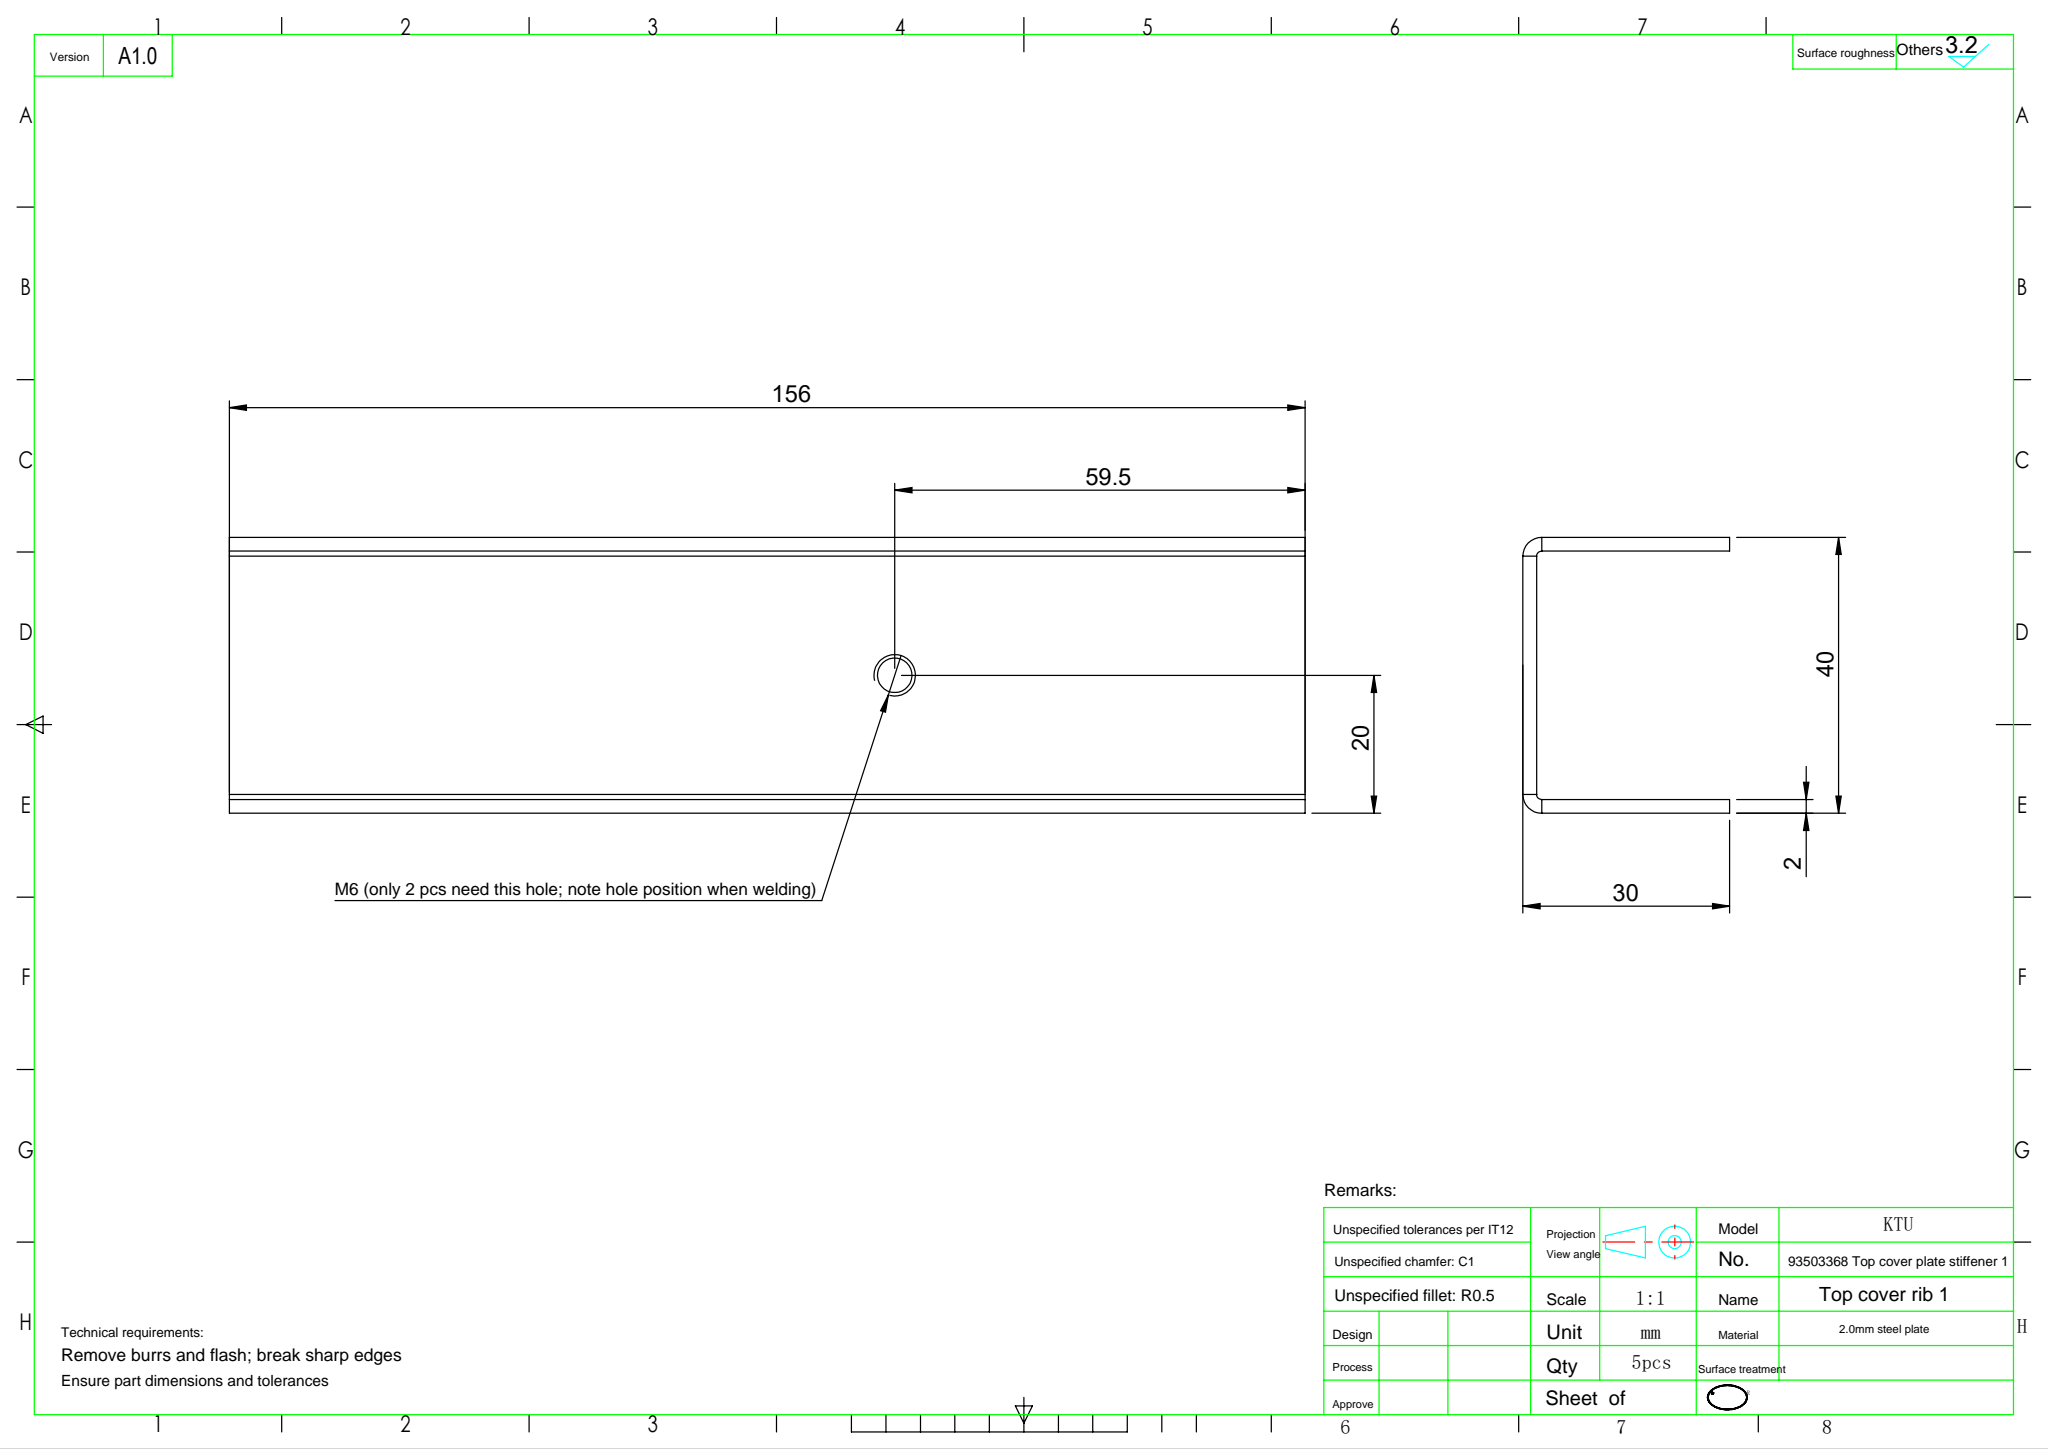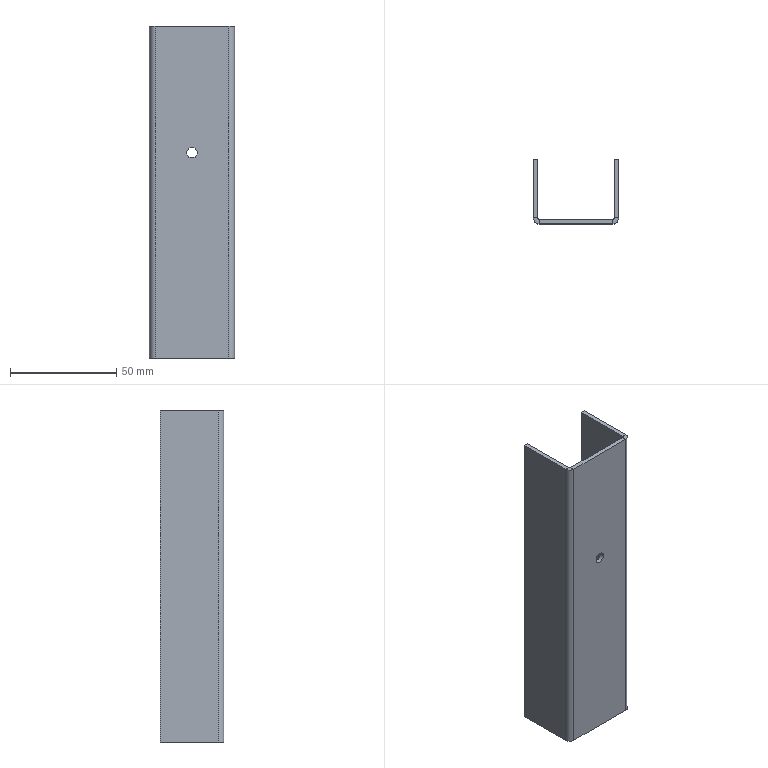Part | SolidWorks | features Cut 1, FlatPattern 1, SMBaseFlange 1, SheetMetal 1 | 1 solid | 24 faces | box 40 x 30 x 156 mm | volume 29448 mm3 | plane 18 | cylinder 6 | commonest cylinder face diameters 1.473 x2 5 x2 5.473 x2
STEP:
#1=CARTESIAN_POINT('',(2.5,-15.,18.5));
#2=VERTEX_POINT('',#1);
#3=CARTESIAN_POINT('',(-2.5,-15.,18.5));
#4=VERTEX_POINT('',#3);
#5=CARTESIAN_POINT('',(0.,-15.,18.5));
#6=DIRECTION('',(0.,1.,0.));
#7=DIRECTION('',(-1.,0.,0.));
#8=AXIS2_PLACEMENT_3D('',#5,#6,#7);
#9=CIRCLE('',#8,2.5);
#10=EDGE_CURVE('',#2,#4,#9,.T.);
#11=ORIENTED_EDGE('',*,*,#10,.F.);
#12=CARTESIAN_POINT('',(2.5,-13.,18.5));
#13=VERTEX_POINT('',#12);
#14=CARTESIAN_POINT('',(2.5,-23.,18.5));
#15=DIRECTION('',(0.,1.,0.));
#16=VECTOR('',#15,1000.);
#17=LINE('',#14,#16);
#18=EDGE_CURVE('',#2,#13,#17,.T.);
#19=ORIENTED_EDGE('',*,*,#18,.T.);
#20=CARTESIAN_POINT('',(-2.5,-13.,18.5));
#21=VERTEX_POINT('',#20);
#22=CARTESIAN_POINT('',(0.,-13.,18.5));
#23=DIRECTION('',(0.,1.,0.));
#24=DIRECTION('',(-1.,0.,0.));
#25=AXIS2_PLACEMENT_3D('',#22,#23,#24);
#26=CIRCLE('',#25,2.5);
#27=EDGE_CURVE('',#13,#21,#26,.T.);
#28=ORIENTED_EDGE('',*,*,#27,.T.);
#29=CARTESIAN_POINT('',(-2.5,-23.,18.5));
#30=DIRECTION('',(0.,1.,0.));
#31=VECTOR('',#30,1000.);
#32=LINE('',#29,#31);
#33=EDGE_CURVE('',#4,#21,#32,.T.);
#34=ORIENTED_EDGE('',*,*,#33,.F.);
#35=EDGE_LOOP('',(#11,#19,#28,#34));
#36=FACE_OUTER_BOUND('',#35,.T.);
#37=CARTESIAN_POINT('',(0.,-23.,18.5));
#38=DIRECTION('',(0.,1.,0.));
#39=DIRECTION('',(-1.,0.,0.));
#40=AXIS2_PLACEMENT_3D('',#37,#38,#39);
#41=CYLINDRICAL_SURFACE('',#40,2.5);
#42=ADVANCED_FACE('',(#36),#41,.F.);
#43=CARTESIAN_POINT('',(-20.,-12.263,78.));
#44=VERTEX_POINT('',#43);
#45=CARTESIAN_POINT('',(-18.,-12.263,78.));
#46=VERTEX_POINT('',#45);
#47=CARTESIAN_POINT('',(-20.,-12.263,78.));
#48=DIRECTION('',(1.,0.,0.));
#49=VECTOR('',#48,1000.);
#50=LINE('',#47,#49);
#51=EDGE_CURVE('',#44,#46,#50,.T.);
#52=ORIENTED_EDGE('',*,*,#51,.F.);
#53=CARTESIAN_POINT('',(-17.263,-15.,78.));
#54=VERTEX_POINT('',#53);
#55=CARTESIAN_POINT('',(-17.263,-12.263,78.));
#56=DIRECTION('',(0.,0.,1.));
#57=DIRECTION('',(-1.,0.,0.));
#58=AXIS2_PLACEMENT_3D('',#55,#56,#57);
#59=CIRCLE('',#58,2.737);
#60=EDGE_CURVE('',#44,#54,#59,.T.);
#61=ORIENTED_EDGE('',*,*,#60,.T.);
#62=CARTESIAN_POINT('',(-17.263,-13.,78.));
#63=VERTEX_POINT('',#62);
#64=CARTESIAN_POINT('',(-17.263,-13.,78.));
#65=DIRECTION('',(0.,-1.,0.));
#66=VECTOR('',#65,1000.);
#67=LINE('',#64,#66);
#68=EDGE_CURVE('',#63,#54,#67,.T.);
#69=ORIENTED_EDGE('',*,*,#68,.F.);
#70=CARTESIAN_POINT('',(-17.263,-12.263,78.));
#71=DIRECTION('',(0.,0.,1.));
#72=DIRECTION('',(1.,0.,0.));
#73=AXIS2_PLACEMENT_3D('',#70,#71,#72);
#74=CIRCLE('',#73,0.7366);
#75=EDGE_CURVE('',#46,#63,#74,.T.);
#76=ORIENTED_EDGE('',*,*,#75,.F.);
#77=EDGE_LOOP('',(#52,#61,#69,#76));
#78=FACE_OUTER_BOUND('',#77,.T.);
#79=CARTESIAN_POINT('',(-20.,-12.263,78.));
#80=DIRECTION('',(0.,0.,1.));
#81=DIRECTION('',(1.,0.,0.));
#82=AXIS2_PLACEMENT_3D('',#79,#80,#81);
#83=PLANE('',#82);
#84=ADVANCED_FACE('',(#78),#83,.T.);
#85=CARTESIAN_POINT('',(-20.,15.,78.));
#86=VERTEX_POINT('',#85);
#87=CARTESIAN_POINT('',(-20.,-15.,78.));
#88=DIRECTION('',(0.,-1.,0.));
#89=VECTOR('',#88,1000.);
#90=LINE('',#87,#89);
#91=EDGE_CURVE('',#86,#44,#90,.T.);
#92=ORIENTED_EDGE('',*,*,#91,.T.);
#93=ORIENTED_EDGE('',*,*,#51,.T.);
#94=CARTESIAN_POINT('',(-18.,15.,78.));
#95=VERTEX_POINT('',#94);
#96=CARTESIAN_POINT('',(-18.,-15.,78.));
#97=DIRECTION('',(0.,-1.,0.));
#98=VECTOR('',#97,1000.);
#99=LINE('',#96,#98);
#100=EDGE_CURVE('',#95,#46,#99,.T.);
#101=ORIENTED_EDGE('',*,*,#100,.F.);
#102=CARTESIAN_POINT('',(-20.,15.,78.));
#103=DIRECTION('',(1.,0.,0.));
#104=VECTOR('',#103,1000.);
#105=LINE('',#102,#104);
#106=EDGE_CURVE('',#86,#95,#105,.T.);
#107=ORIENTED_EDGE('',*,*,#106,.F.);
#108=EDGE_LOOP('',(#92,#93,#101,#107));
#109=FACE_OUTER_BOUND('',#108,.T.);
#110=CARTESIAN_POINT('',(-17.263,-13.,78.));
#111=DIRECTION('',(0.,0.,1.));
#112=DIRECTION('',(1.,0.,0.));
#113=AXIS2_PLACEMENT_3D('',#110,#111,#112);
#114=PLANE('',#113);
#115=ADVANCED_FACE('',(#109),#114,.T.);
#116=CARTESIAN_POINT('',(-17.263,-15.,-78.));
#117=VERTEX_POINT('',#116);
#118=CARTESIAN_POINT('',(-17.263,-13.,-78.));
#119=VERTEX_POINT('',#118);
#120=CARTESIAN_POINT('',(-17.263,-15.,-78.));
#121=DIRECTION('',(0.,1.,0.));
#122=VECTOR('',#121,1000.);
#123=LINE('',#120,#122);
#124=EDGE_CURVE('',#117,#119,#123,.T.);
#125=ORIENTED_EDGE('',*,*,#124,.F.);
#126=CARTESIAN_POINT('',(-20.,-12.263,-78.));
#127=VERTEX_POINT('',#126);
#128=CARTESIAN_POINT('',(-17.263,-12.263,-78.));
#129=DIRECTION('',(0.,0.,1.));
#130=DIRECTION('',(-1.,0.,0.));
#131=AXIS2_PLACEMENT_3D('',#128,#129,#130);
#132=CIRCLE('',#131,2.737);
#133=EDGE_CURVE('',#127,#117,#132,.T.);
#134=ORIENTED_EDGE('',*,*,#133,.F.);
#135=CARTESIAN_POINT('',(-18.,-12.263,-78.));
#136=VERTEX_POINT('',#135);
#137=CARTESIAN_POINT('',(-18.,-12.263,-78.));
#138=DIRECTION('',(-1.,0.,0.));
#139=VECTOR('',#138,1000.);
#140=LINE('',#137,#139);
#141=EDGE_CURVE('',#136,#127,#140,.T.);
#142=ORIENTED_EDGE('',*,*,#141,.F.);
#143=CARTESIAN_POINT('',(-17.263,-12.263,-78.));
#144=DIRECTION('',(0.,0.,1.));
#145=DIRECTION('',(1.,0.,0.));
#146=AXIS2_PLACEMENT_3D('',#143,#144,#145);
#147=CIRCLE('',#146,0.7366);
#148=EDGE_CURVE('',#136,#119,#147,.T.);
#149=ORIENTED_EDGE('',*,*,#148,.T.);
#150=EDGE_LOOP('',(#125,#134,#142,#149));
#151=FACE_OUTER_BOUND('',#150,.T.);
#152=CARTESIAN_POINT('',(-17.263,-15.,-78.));
#153=DIRECTION('',(0.,0.,-1.));
#154=DIRECTION('',(-1.,0.,0.));
#155=AXIS2_PLACEMENT_3D('',#152,#153,#154);
#156=PLANE('',#155);
#157=ADVANCED_FACE('',(#151),#156,.T.);
#158=CARTESIAN_POINT('',(17.263,-15.,-78.));
#159=VERTEX_POINT('',#158);
#160=CARTESIAN_POINT('',(20.,-15.,-78.));
#161=DIRECTION('',(1.,0.,0.));
#162=VECTOR('',#161,1000.);
#163=LINE('',#160,#162);
#164=EDGE_CURVE('',#117,#159,#163,.T.);
#165=ORIENTED_EDGE('',*,*,#164,.F.);
#166=ORIENTED_EDGE('',*,*,#124,.T.);
#167=CARTESIAN_POINT('',(17.263,-13.,-78.));
#168=VERTEX_POINT('',#167);
#169=CARTESIAN_POINT('',(20.,-13.,-78.));
#170=DIRECTION('',(1.,0.,0.));
#171=VECTOR('',#170,1000.);
#172=LINE('',#169,#171);
#173=EDGE_CURVE('',#119,#168,#172,.T.);
#174=ORIENTED_EDGE('',*,*,#173,.T.);
#175=CARTESIAN_POINT('',(17.263,-13.,-78.));
#176=DIRECTION('',(0.,-1.,0.));
#177=VECTOR('',#176,1000.);
#178=LINE('',#175,#177);
#179=EDGE_CURVE('',#168,#159,#178,.T.);
#180=ORIENTED_EDGE('',*,*,#179,.T.);
#181=EDGE_LOOP('',(#165,#166,#174,#180));
#182=FACE_OUTER_BOUND('',#181,.T.);
#183=CARTESIAN_POINT('',(-18.,-12.263,-78.));
#184=DIRECTION('',(0.,0.,-1.));
#185=DIRECTION('',(-1.,0.,0.));
#186=AXIS2_PLACEMENT_3D('',#183,#184,#185);
#187=PLANE('',#186);
#188=ADVANCED_FACE('',(#182),#187,.T.);
#189=CARTESIAN_POINT('',(17.263,-15.,78.));
#190=VERTEX_POINT('',#189);
#191=CARTESIAN_POINT('',(17.263,-13.,78.));
#192=VERTEX_POINT('',#191);
#193=CARTESIAN_POINT('',(17.263,-15.,78.));
#194=DIRECTION('',(0.,1.,0.));
#195=VECTOR('',#194,1000.);
#196=LINE('',#193,#195);
#197=EDGE_CURVE('',#190,#192,#196,.T.);
#198=ORIENTED_EDGE('',*,*,#197,.F.);
#199=CARTESIAN_POINT('',(20.,-12.263,78.));
#200=VERTEX_POINT('',#199);
#201=CARTESIAN_POINT('',(17.263,-12.263,78.));
#202=DIRECTION('',(0.,0.,1.));
#203=DIRECTION('',(-1.,0.,0.));
#204=AXIS2_PLACEMENT_3D('',#201,#202,#203);
#205=CIRCLE('',#204,2.737);
#206=EDGE_CURVE('',#190,#200,#205,.T.);
#207=ORIENTED_EDGE('',*,*,#206,.T.);
#208=CARTESIAN_POINT('',(18.,-12.263,78.));
#209=VERTEX_POINT('',#208);
#210=CARTESIAN_POINT('',(18.,-12.263,78.));
#211=DIRECTION('',(1.,0.,0.));
#212=VECTOR('',#211,1000.);
#213=LINE('',#210,#212);
#214=EDGE_CURVE('',#209,#200,#213,.T.);
#215=ORIENTED_EDGE('',*,*,#214,.F.);
#216=CARTESIAN_POINT('',(17.263,-12.263,78.));
#217=DIRECTION('',(0.,0.,1.));
#218=DIRECTION('',(1.,0.,0.));
#219=AXIS2_PLACEMENT_3D('',#216,#217,#218);
#220=CIRCLE('',#219,0.7366);
#221=EDGE_CURVE('',#192,#209,#220,.T.);
#222=ORIENTED_EDGE('',*,*,#221,.F.);
#223=EDGE_LOOP('',(#198,#207,#215,#222));
#224=FACE_OUTER_BOUND('',#223,.T.);
#225=CARTESIAN_POINT('',(17.263,-15.,78.));
#226=DIRECTION('',(0.,0.,1.));
#227=DIRECTION('',(1.,0.,0.));
#228=AXIS2_PLACEMENT_3D('',#225,#226,#227);
#229=PLANE('',#228);
#230=ADVANCED_FACE('',(#224),#229,.T.);
#231=CARTESIAN_POINT('',(20.,-15.,78.));
#232=DIRECTION('',(1.,0.,0.));
#233=VECTOR('',#232,1000.);
#234=LINE('',#231,#233);
#235=EDGE_CURVE('',#54,#190,#234,.T.);
#236=ORIENTED_EDGE('',*,*,#235,.T.);
#237=ORIENTED_EDGE('',*,*,#197,.T.);
#238=CARTESIAN_POINT('',(20.,-13.,78.));
#239=DIRECTION('',(1.,0.,0.));
#240=VECTOR('',#239,1000.);
#241=LINE('',#238,#240);
#242=EDGE_CURVE('',#63,#192,#241,.T.);
#243=ORIENTED_EDGE('',*,*,#242,.F.);
#244=ORIENTED_EDGE('',*,*,#68,.T.);
#245=EDGE_LOOP('',(#236,#237,#243,#244));
#246=FACE_OUTER_BOUND('',#245,.T.);
#247=CARTESIAN_POINT('',(18.,-12.263,78.));
#248=DIRECTION('',(0.,0.,1.));
#249=DIRECTION('',(1.,0.,0.));
#250=AXIS2_PLACEMENT_3D('',#247,#248,#249);
#251=PLANE('',#250);
#252=ADVANCED_FACE('',(#246),#251,.T.);
#253=CARTESIAN_POINT('',(20.,-12.263,-78.));
#254=VERTEX_POINT('',#253);
#255=CARTESIAN_POINT('',(18.,-12.263,-78.));
#256=VERTEX_POINT('',#255);
#257=CARTESIAN_POINT('',(20.,-12.263,-78.));
#258=DIRECTION('',(-1.,0.,0.));
#259=VECTOR('',#258,1000.);
#260=LINE('',#257,#259);
#261=EDGE_CURVE('',#254,#256,#260,.T.);
#262=ORIENTED_EDGE('',*,*,#261,.F.);
#263=CARTESIAN_POINT('',(17.263,-12.263,-78.));
#264=DIRECTION('',(0.,0.,1.));
#265=DIRECTION('',(-1.,0.,0.));
#266=AXIS2_PLACEMENT_3D('',#263,#264,#265);
#267=CIRCLE('',#266,2.737);
#268=EDGE_CURVE('',#159,#254,#267,.T.);
#269=ORIENTED_EDGE('',*,*,#268,.F.);
#270=ORIENTED_EDGE('',*,*,#179,.F.);
#271=CARTESIAN_POINT('',(17.263,-12.263,-78.));
#272=DIRECTION('',(0.,0.,1.));
#273=DIRECTION('',(1.,0.,0.));
#274=AXIS2_PLACEMENT_3D('',#271,#272,#273);
#275=CIRCLE('',#274,0.7366);
#276=EDGE_CURVE('',#168,#256,#275,.T.);
#277=ORIENTED_EDGE('',*,*,#276,.T.);
#278=EDGE_LOOP('',(#262,#269,#270,#277));
#279=FACE_OUTER_BOUND('',#278,.T.);
#280=CARTESIAN_POINT('',(20.,-12.263,-78.));
#281=DIRECTION('',(0.,0.,-1.));
#282=DIRECTION('',(-1.,0.,0.));
#283=AXIS2_PLACEMENT_3D('',#280,#281,#282);
#284=PLANE('',#283);
#285=ADVANCED_FACE('',(#279),#284,.T.);
#286=CARTESIAN_POINT('',(20.,15.,-78.));
#287=VERTEX_POINT('',#286);
#288=CARTESIAN_POINT('',(20.,-15.,-78.));
#289=DIRECTION('',(0.,1.,0.));
#290=VECTOR('',#289,1000.);
#291=LINE('',#288,#290);
#292=EDGE_CURVE('',#254,#287,#291,.T.);
#293=ORIENTED_EDGE('',*,*,#292,.F.);
#294=ORIENTED_EDGE('',*,*,#261,.T.);
#295=CARTESIAN_POINT('',(18.,15.,-78.));
#296=VERTEX_POINT('',#295);
#297=CARTESIAN_POINT('',(18.,-15.,-78.));
#298=DIRECTION('',(0.,1.,0.));
#299=VECTOR('',#298,1000.);
#300=LINE('',#297,#299);
#301=EDGE_CURVE('',#256,#296,#300,.T.);
#302=ORIENTED_EDGE('',*,*,#301,.T.);
#303=CARTESIAN_POINT('',(18.,15.,-78.));
#304=DIRECTION('',(1.,0.,0.));
#305=VECTOR('',#304,1000.);
#306=LINE('',#303,#305);
#307=EDGE_CURVE('',#296,#287,#306,.T.);
#308=ORIENTED_EDGE('',*,*,#307,.T.);
#309=EDGE_LOOP('',(#293,#294,#302,#308));
#310=FACE_OUTER_BOUND('',#309,.T.);
#311=CARTESIAN_POINT('',(17.263,-13.,-78.));
#312=DIRECTION('',(0.,0.,-1.));
#313=DIRECTION('',(-1.,0.,0.));
#314=AXIS2_PLACEMENT_3D('',#311,#312,#313);
#315=PLANE('',#314);
#316=ADVANCED_FACE('',(#310),#315,.T.);
#317=ORIENTED_EDGE('',*,*,#292,.T.);
#318=CARTESIAN_POINT('',(20.,15.,78.));
#319=VERTEX_POINT('',#318);
#320=CARTESIAN_POINT('',(20.,15.,78.));
#321=DIRECTION('',(0.,0.,-1.));
#322=VECTOR('',#321,1000.);
#323=LINE('',#320,#322);
#324=EDGE_CURVE('',#319,#287,#323,.T.);
#325=ORIENTED_EDGE('',*,*,#324,.F.);
#326=CARTESIAN_POINT('',(20.,-15.,78.));
#327=DIRECTION('',(0.,1.,0.));
#328=VECTOR('',#327,1000.);
#329=LINE('',#326,#328);
#330=EDGE_CURVE('',#200,#319,#329,.T.);
#331=ORIENTED_EDGE('',*,*,#330,.F.);
#332=CARTESIAN_POINT('',(20.,-12.263,78.));
#333=DIRECTION('',(0.,0.,-1.));
#334=VECTOR('',#333,1000.);
#335=LINE('',#332,#334);
#336=EDGE_CURVE('',#200,#254,#335,.T.);
#337=ORIENTED_EDGE('',*,*,#336,.T.);
#338=EDGE_LOOP('',(#317,#325,#331,#337));
#339=FACE_OUTER_BOUND('',#338,.T.);
#340=CARTESIAN_POINT('',(20.,-15.,78.));
#341=DIRECTION('',(-1.,0.,0.));
#342=DIRECTION('',(0.,0.,1.));
#343=AXIS2_PLACEMENT_3D('',#340,#341,#342);
#344=PLANE('',#343);
#345=ADVANCED_FACE('',(#339),#344,.F.);
#346=ORIENTED_EDGE('',*,*,#307,.F.);
#347=CARTESIAN_POINT('',(18.,15.,78.));
#348=VERTEX_POINT('',#347);
#349=CARTESIAN_POINT('',(18.,15.,78.));
#350=DIRECTION('',(0.,0.,-1.));
#351=VECTOR('',#350,1000.);
#352=LINE('',#349,#351);
#353=EDGE_CURVE('',#348,#296,#352,.T.);
#354=ORIENTED_EDGE('',*,*,#353,.F.);
#355=CARTESIAN_POINT('',(18.,15.,78.));
#356=DIRECTION('',(1.,0.,0.));
#357=VECTOR('',#356,1000.);
#358=LINE('',#355,#357);
#359=EDGE_CURVE('',#348,#319,#358,.T.);
#360=ORIENTED_EDGE('',*,*,#359,.T.);
#361=ORIENTED_EDGE('',*,*,#324,.T.);
#362=EDGE_LOOP('',(#346,#354,#360,#361));
#363=FACE_OUTER_BOUND('',#362,.T.);
#364=CARTESIAN_POINT('',(18.,15.,78.));
#365=DIRECTION('',(0.,1.,0.));
#366=DIRECTION('',(-1.,0.,0.));
#367=AXIS2_PLACEMENT_3D('',#364,#365,#366);
#368=PLANE('',#367);
#369=ADVANCED_FACE('',(#363),#368,.T.);
#370=ORIENTED_EDGE('',*,*,#301,.F.);
#371=CARTESIAN_POINT('',(18.,-12.263,78.));
#372=DIRECTION('',(0.,0.,-1.));
#373=VECTOR('',#372,1000.);
#374=LINE('',#371,#373);
#375=EDGE_CURVE('',#209,#256,#374,.T.);
#376=ORIENTED_EDGE('',*,*,#375,.F.);
#377=CARTESIAN_POINT('',(18.,-15.,78.));
#378=DIRECTION('',(0.,1.,0.));
#379=VECTOR('',#378,1000.);
#380=LINE('',#377,#379);
#381=EDGE_CURVE('',#209,#348,#380,.T.);
#382=ORIENTED_EDGE('',*,*,#381,.T.);
#383=ORIENTED_EDGE('',*,*,#353,.T.);
#384=EDGE_LOOP('',(#370,#376,#382,#383));
#385=FACE_OUTER_BOUND('',#384,.T.);
#386=CARTESIAN_POINT('',(18.,-15.,78.));
#387=DIRECTION('',(-1.,0.,0.));
#388=DIRECTION('',(0.,0.,1.));
#389=AXIS2_PLACEMENT_3D('',#386,#387,#388);
#390=PLANE('',#389);
#391=ADVANCED_FACE('',(#385),#390,.T.);
#392=ORIENTED_EDGE('',*,*,#276,.F.);
#393=CARTESIAN_POINT('',(17.263,-13.,78.));
#394=DIRECTION('',(0.,0.,-1.));
#395=VECTOR('',#394,1000.);
#396=LINE('',#393,#395);
#397=EDGE_CURVE('',#192,#168,#396,.T.);
#398=ORIENTED_EDGE('',*,*,#397,.F.);
#399=ORIENTED_EDGE('',*,*,#221,.T.);
#400=ORIENTED_EDGE('',*,*,#375,.T.);
#401=EDGE_LOOP('',(#392,#398,#399,#400));
#402=FACE_OUTER_BOUND('',#401,.T.);
#403=CARTESIAN_POINT('',(17.263,-12.263,78.));
#404=DIRECTION('',(0.,0.,-1.));
#405=DIRECTION('',(-1.,0.,0.));
#406=AXIS2_PLACEMENT_3D('',#403,#404,#405);
#407=CYLINDRICAL_SURFACE('',#406,0.7366);
#408=ADVANCED_FACE('',(#402),#407,.F.);
#409=CARTESIAN_POINT('',(0.,-13.,18.5));
#410=DIRECTION('',(0.,1.,0.));
#411=DIRECTION('',(-1.,0.,0.));
#412=AXIS2_PLACEMENT_3D('',#409,#410,#411);
#413=CIRCLE('',#412,2.5);
#414=EDGE_CURVE('',#21,#13,#413,.T.);
#415=ORIENTED_EDGE('',*,*,#414,.F.);
#416=ORIENTED_EDGE('',*,*,#27,.F.);
#417=EDGE_LOOP('',(#415,#416));
#418=FACE_BOUND('',#417,.T.);
#419=ORIENTED_EDGE('',*,*,#173,.F.);
#420=CARTESIAN_POINT('',(-17.263,-13.,78.));
#421=DIRECTION('',(0.,0.,-1.));
#422=VECTOR('',#421,1000.);
#423=LINE('',#420,#422);
#424=EDGE_CURVE('',#63,#119,#423,.T.);
#425=ORIENTED_EDGE('',*,*,#424,.F.);
#426=ORIENTED_EDGE('',*,*,#242,.T.);
#427=ORIENTED_EDGE('',*,*,#397,.T.);
#428=EDGE_LOOP('',(#419,#425,#426,#427));
#429=FACE_OUTER_BOUND('',#428,.T.);
#430=CARTESIAN_POINT('',(20.,-13.,78.));
#431=DIRECTION('',(0.,1.,0.));
#432=DIRECTION('',(-1.,0.,0.));
#433=AXIS2_PLACEMENT_3D('',#430,#431,#432);
#434=PLANE('',#433);
#435=ADVANCED_FACE('',(#418,#429),#434,.T.);
#436=ORIENTED_EDGE('',*,*,#148,.F.);
#437=CARTESIAN_POINT('',(-18.,-12.263,78.));
#438=DIRECTION('',(0.,0.,-1.));
#439=VECTOR('',#438,1000.);
#440=LINE('',#437,#439);
#441=EDGE_CURVE('',#46,#136,#440,.T.);
#442=ORIENTED_EDGE('',*,*,#441,.F.);
#443=ORIENTED_EDGE('',*,*,#75,.T.);
#444=ORIENTED_EDGE('',*,*,#424,.T.);
#445=EDGE_LOOP('',(#436,#442,#443,#444));
#446=FACE_OUTER_BOUND('',#445,.T.);
#447=CARTESIAN_POINT('',(-17.263,-12.263,78.));
#448=DIRECTION('',(0.,0.,-1.));
#449=DIRECTION('',(-1.,0.,0.));
#450=AXIS2_PLACEMENT_3D('',#447,#448,#449);
#451=CYLINDRICAL_SURFACE('',#450,0.7366);
#452=ADVANCED_FACE('',(#446),#451,.F.);
#453=CARTESIAN_POINT('',(-18.,15.,-78.));
#454=VERTEX_POINT('',#453);
#455=CARTESIAN_POINT('',(-18.,-15.,-78.));
#456=DIRECTION('',(0.,-1.,0.));
#457=VECTOR('',#456,1000.);
#458=LINE('',#455,#457);
#459=EDGE_CURVE('',#454,#136,#458,.T.);
#460=ORIENTED_EDGE('',*,*,#459,.F.);
#461=CARTESIAN_POINT('',(-18.,15.,78.));
#462=DIRECTION('',(0.,0.,-1.));
#463=VECTOR('',#462,1000.);
#464=LINE('',#461,#463);
#465=EDGE_CURVE('',#95,#454,#464,.T.);
#466=ORIENTED_EDGE('',*,*,#465,.F.);
#467=ORIENTED_EDGE('',*,*,#100,.T.);
#468=ORIENTED_EDGE('',*,*,#441,.T.);
#469=EDGE_LOOP('',(#460,#466,#467,#468));
#470=FACE_OUTER_BOUND('',#469,.T.);
#471=CARTESIAN_POINT('',(-18.,-15.,78.));
#472=DIRECTION('',(1.,0.,0.));
#473=DIRECTION('',(0.,0.,-1.));
#474=AXIS2_PLACEMENT_3D('',#471,#472,#473);
#475=PLANE('',#474);
#476=ADVANCED_FACE('',(#470),#475,.T.);
#477=CARTESIAN_POINT('',(-20.,15.,-78.));
#478=VERTEX_POINT('',#477);
#479=CARTESIAN_POINT('',(-20.,15.,-78.));
#480=DIRECTION('',(1.,0.,0.));
#481=VECTOR('',#480,1000.);
#482=LINE('',#479,#481);
#483=EDGE_CURVE('',#478,#454,#482,.T.);
#484=ORIENTED_EDGE('',*,*,#483,.F.);
#485=CARTESIAN_POINT('',(-20.,15.,78.));
#486=DIRECTION('',(0.,0.,-1.));
#487=VECTOR('',#486,1000.);
#488=LINE('',#485,#487);
#489=EDGE_CURVE('',#86,#478,#488,.T.);
#490=ORIENTED_EDGE('',*,*,#489,.F.);
#491=ORIENTED_EDGE('',*,*,#106,.T.);
#492=ORIENTED_EDGE('',*,*,#465,.T.);
#493=EDGE_LOOP('',(#484,#490,#491,#492));
#494=FACE_OUTER_BOUND('',#493,.T.);
#495=CARTESIAN_POINT('',(-20.,15.,78.));
#496=DIRECTION('',(0.,1.,0.));
#497=DIRECTION('',(-1.,0.,0.));
#498=AXIS2_PLACEMENT_3D('',#495,#496,#497);
#499=PLANE('',#498);
#500=ADVANCED_FACE('',(#494),#499,.T.);
#501=CARTESIAN_POINT('',(-20.,-15.,-78.));
#502=DIRECTION('',(0.,-1.,0.));
#503=VECTOR('',#502,1000.);
#504=LINE('',#501,#503);
#505=EDGE_CURVE('',#478,#127,#504,.T.);
#506=ORIENTED_EDGE('',*,*,#505,.T.);
#507=CARTESIAN_POINT('',(-20.,-12.263,78.));
#508=DIRECTION('',(0.,0.,-1.));
#509=VECTOR('',#508,1000.);
#510=LINE('',#507,#509);
#511=EDGE_CURVE('',#44,#127,#510,.T.);
#512=ORIENTED_EDGE('',*,*,#511,.F.);
#513=ORIENTED_EDGE('',*,*,#91,.F.);
#514=ORIENTED_EDGE('',*,*,#489,.T.);
#515=EDGE_LOOP('',(#506,#512,#513,#514));
#516=FACE_OUTER_BOUND('',#515,.T.);
#517=CARTESIAN_POINT('',(-20.,-15.,78.));
#518=DIRECTION('',(1.,0.,0.));
#519=DIRECTION('',(0.,0.,-1.));
#520=AXIS2_PLACEMENT_3D('',#517,#518,#519);
#521=PLANE('',#520);
#522=ADVANCED_FACE('',(#516),#521,.F.);
#523=ORIENTED_EDGE('',*,*,#133,.T.);
#524=CARTESIAN_POINT('',(-17.263,-15.,78.));
#525=DIRECTION('',(0.,0.,-1.));
#526=VECTOR('',#525,1000.);
#527=LINE('',#524,#526);
#528=EDGE_CURVE('',#54,#117,#527,.T.);
#529=ORIENTED_EDGE('',*,*,#528,.F.);
#530=ORIENTED_EDGE('',*,*,#60,.F.);
#531=ORIENTED_EDGE('',*,*,#511,.T.);
#532=EDGE_LOOP('',(#523,#529,#530,#531));
#533=FACE_OUTER_BOUND('',#532,.T.);
#534=CARTESIAN_POINT('',(-17.263,-12.263,78.));
#535=DIRECTION('',(0.,0.,-1.));
#536=DIRECTION('',(-1.,0.,0.));
#537=AXIS2_PLACEMENT_3D('',#534,#535,#536);
#538=CYLINDRICAL_SURFACE('',#537,2.737);
#539=ADVANCED_FACE('',(#533),#538,.T.);
#540=CARTESIAN_POINT('',(0.,-15.,18.5));
#541=DIRECTION('',(0.,1.,0.));
#542=DIRECTION('',(-1.,0.,0.));
#543=AXIS2_PLACEMENT_3D('',#540,#541,#542);
#544=CIRCLE('',#543,2.5);
#545=EDGE_CURVE('',#4,#2,#544,.T.);
#546=ORIENTED_EDGE('',*,*,#545,.T.);
#547=ORIENTED_EDGE('',*,*,#10,.T.);
#548=EDGE_LOOP('',(#546,#547));
#549=FACE_BOUND('',#548,.T.);
#550=ORIENTED_EDGE('',*,*,#164,.T.);
#551=CARTESIAN_POINT('',(17.263,-15.,78.));
#552=DIRECTION('',(0.,0.,-1.));
#553=VECTOR('',#552,1000.);
#554=LINE('',#551,#553);
#555=EDGE_CURVE('',#190,#159,#554,.T.);
#556=ORIENTED_EDGE('',*,*,#555,.F.);
#557=ORIENTED_EDGE('',*,*,#235,.F.);
#558=ORIENTED_EDGE('',*,*,#528,.T.);
#559=EDGE_LOOP('',(#550,#556,#557,#558));
#560=FACE_OUTER_BOUND('',#559,.T.);
#561=CARTESIAN_POINT('',(20.,-15.,78.));
#562=DIRECTION('',(0.,1.,0.));
#563=DIRECTION('',(-1.,0.,0.));
#564=AXIS2_PLACEMENT_3D('',#561,#562,#563);
#565=PLANE('',#564);
#566=ADVANCED_FACE('',(#549,#560),#565,.F.);
#567=ORIENTED_EDGE('',*,*,#268,.T.);
#568=ORIENTED_EDGE('',*,*,#336,.F.);
#569=ORIENTED_EDGE('',*,*,#206,.F.);
#570=ORIENTED_EDGE('',*,*,#555,.T.);
#571=EDGE_LOOP('',(#567,#568,#569,#570));
#572=FACE_OUTER_BOUND('',#571,.T.);
#573=CARTESIAN_POINT('',(17.263,-12.263,78.));
#574=DIRECTION('',(0.,0.,-1.));
#575=DIRECTION('',(-1.,0.,0.));
#576=AXIS2_PLACEMENT_3D('',#573,#574,#575);
#577=CYLINDRICAL_SURFACE('',#576,2.737);
#578=ADVANCED_FACE('',(#572),#577,.T.);
#579=ORIENTED_EDGE('',*,*,#330,.T.);
#580=ORIENTED_EDGE('',*,*,#359,.F.);
#581=ORIENTED_EDGE('',*,*,#381,.F.);
#582=ORIENTED_EDGE('',*,*,#214,.T.);
#583=EDGE_LOOP('',(#579,#580,#581,#582));
#584=FACE_OUTER_BOUND('',#583,.T.);
#585=CARTESIAN_POINT('',(17.263,-12.263,78.));
#586=DIRECTION('',(0.,0.,1.));
#587=DIRECTION('',(1.,0.,0.));
#588=AXIS2_PLACEMENT_3D('',#585,#586,#587);
#589=PLANE('',#588);
#590=ADVANCED_FACE('',(#584),#589,.T.);
#591=ORIENTED_EDGE('',*,*,#459,.T.);
#592=ORIENTED_EDGE('',*,*,#141,.T.);
#593=ORIENTED_EDGE('',*,*,#505,.F.);
#594=ORIENTED_EDGE('',*,*,#483,.T.);
#595=EDGE_LOOP('',(#591,#592,#593,#594));
#596=FACE_OUTER_BOUND('',#595,.T.);
#597=CARTESIAN_POINT('',(17.263,-12.263,-78.));
#598=DIRECTION('',(0.,0.,1.));
#599=DIRECTION('',(1.,0.,0.));
#600=AXIS2_PLACEMENT_3D('',#597,#598,#599);
#601=PLANE('',#600);
#602=ADVANCED_FACE('',(#596),#601,.F.);
#603=ORIENTED_EDGE('',*,*,#18,.F.);
#604=ORIENTED_EDGE('',*,*,#545,.F.);
#605=ORIENTED_EDGE('',*,*,#33,.T.);
#606=ORIENTED_EDGE('',*,*,#414,.T.);
#607=EDGE_LOOP('',(#603,#604,#605,#606));
#608=FACE_OUTER_BOUND('',#607,.T.);
#609=CARTESIAN_POINT('',(0.,-23.,18.5));
#610=DIRECTION('',(0.,1.,0.));
#611=DIRECTION('',(-1.,0.,0.));
#612=AXIS2_PLACEMENT_3D('',#609,#610,#611);
#613=CYLINDRICAL_SURFACE('',#612,2.5);
#614=ADVANCED_FACE('',(#608),#613,.F.);
#615=CLOSED_SHELL('',(#42,#84,#115,#157,#188,#230,#252,#285,#316,#345,#369,#391,#408,#435,#452,#476,#500,#522,#539,#566,#578,#590,#602,#614));
#616=MANIFOLD_SOLID_BREP('',#615);
#617=CARTESIAN_POINT('',(0.,0.,0.));
#618=DIRECTION('',(0.,0.,1.));
#619=DIRECTION('',(1.,0.,0.));
#620=AXIS2_PLACEMENT_3D('',#617,#618,#619);
#621=(LENGTH_UNIT()NAMED_UNIT(*)SI_UNIT(.MILLI.,.METRE.));
#622=UNCERTAINTY_MEASURE_WITH_UNIT(LENGTH_MEASURE(0.00001),#621,'','');
#623=(NAMED_UNIT(*)PLANE_ANGLE_UNIT()SI_UNIT($,.RADIAN.));
#624=(NAMED_UNIT(*)SI_UNIT($,.STERADIAN.)SOLID_ANGLE_UNIT());
#625=(GEOMETRIC_REPRESENTATION_CONTEXT(3)GLOBAL_UNCERTAINTY_ASSIGNED_CONTEXT((#622))GLOBAL_UNIT_ASSIGNED_CONTEXT((#621,#623,#624))REPRESENTATION_CONTEXT('',''));
#626=ADVANCED_BREP_SHAPE_REPRESENTATION('',(#616,#620),#625);